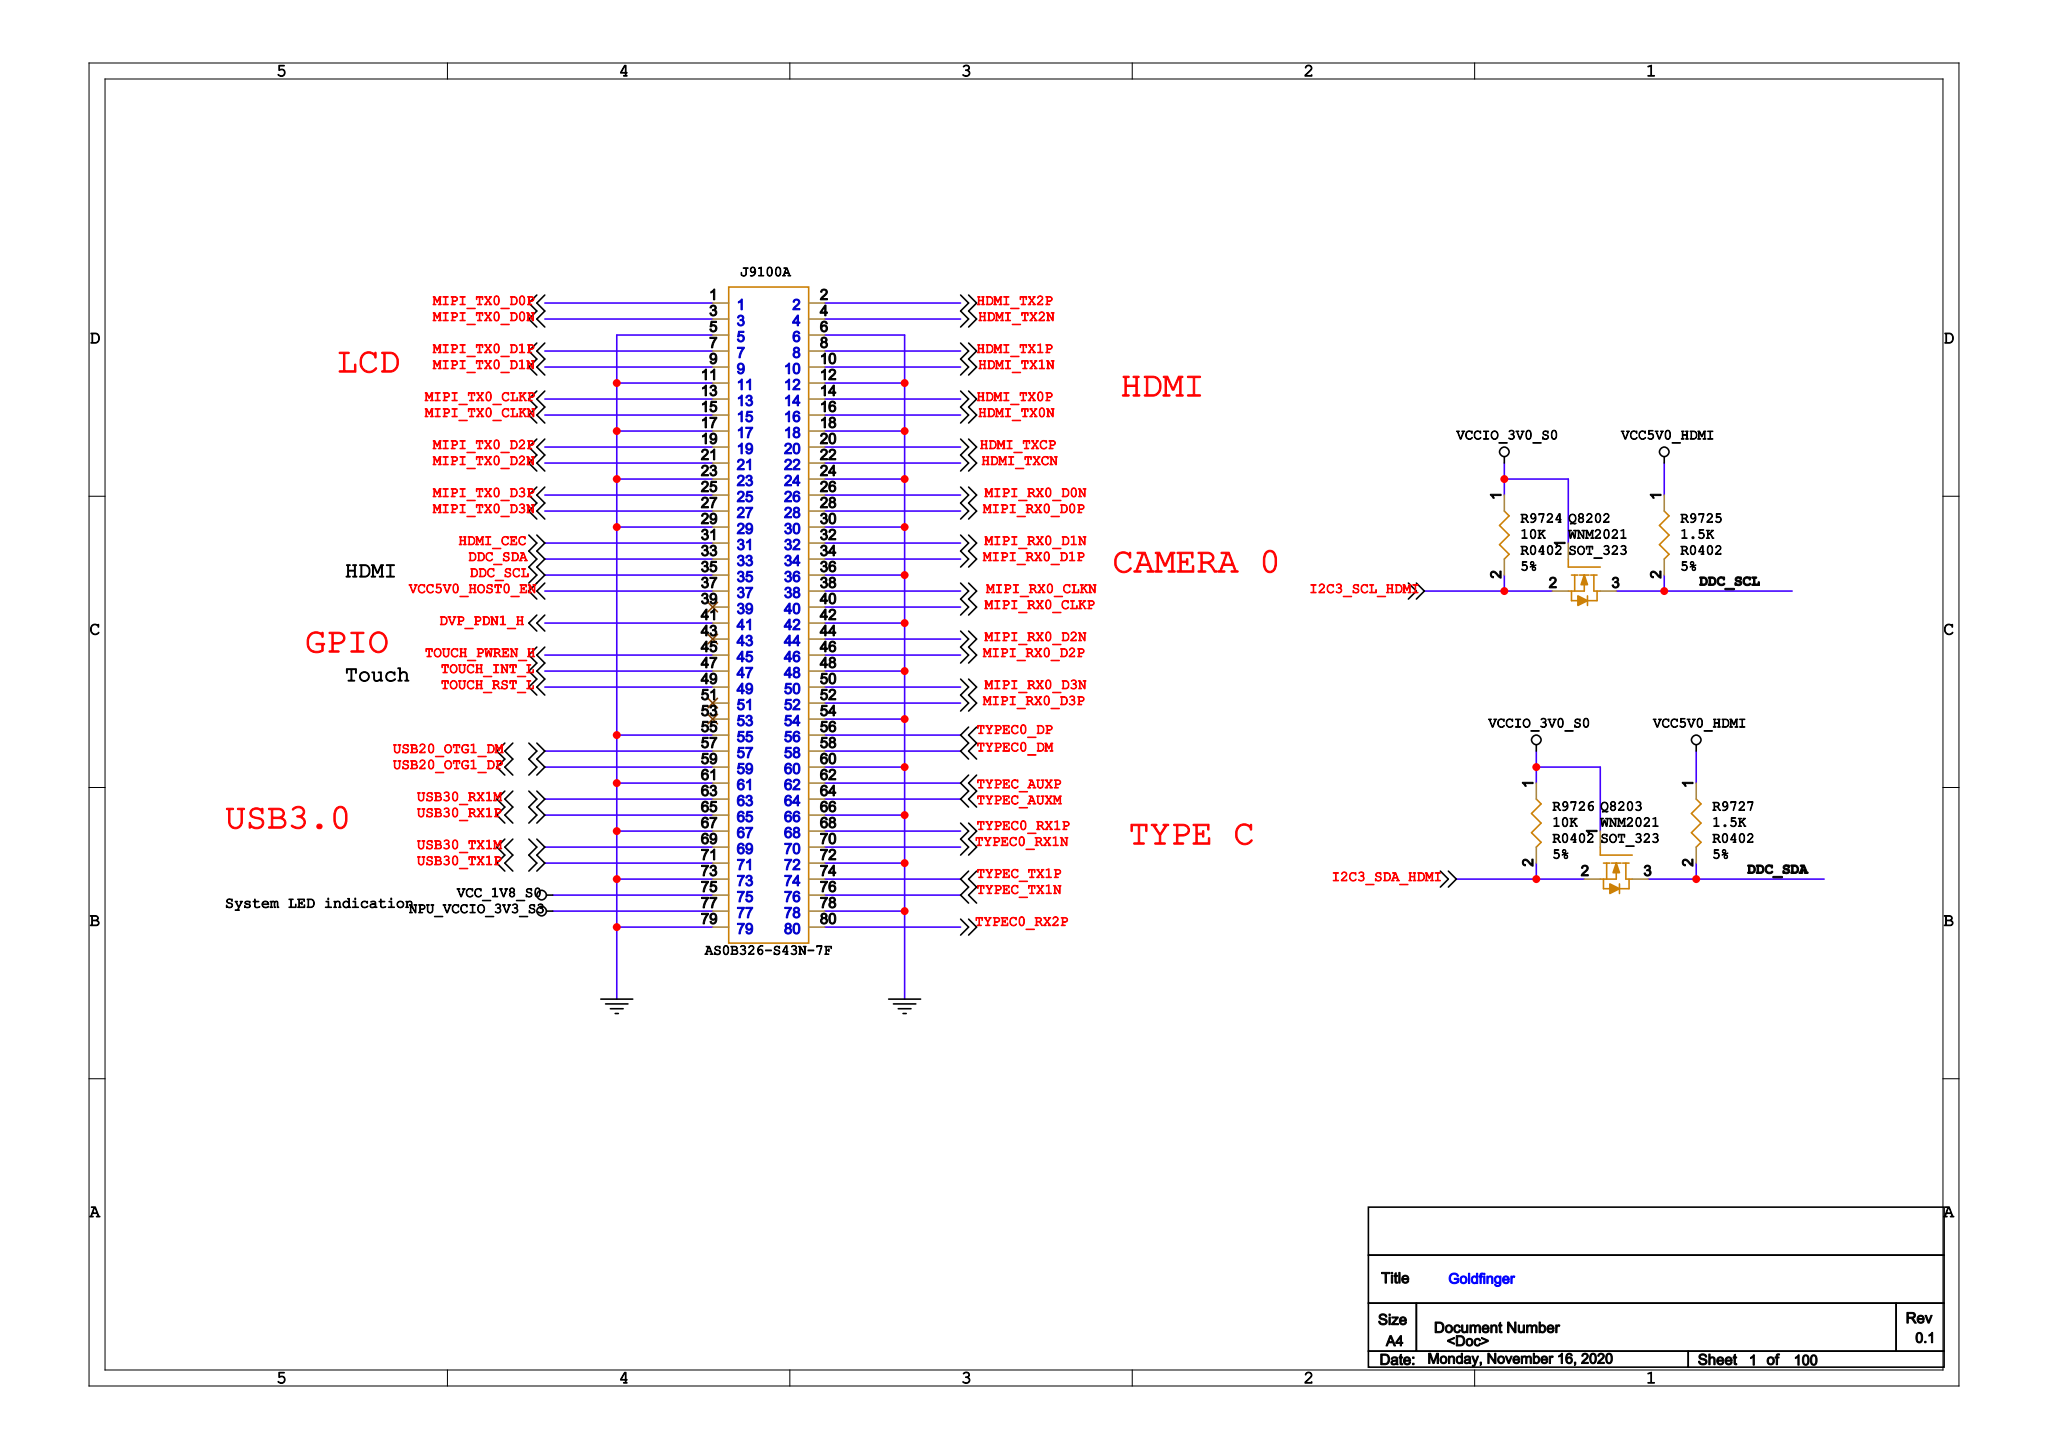Circuit board | Cadence Allegro | 749 parts | 717 nets | one sheet of the schematic
Parts on this sheet (reference | value | footprint):
J9100 | AS0B326-S43N-7F | MXM_230P_0P5
Q8202 | WNM2021 | SOT_323
Q8203 | WNM2021 | SOT_323
R9724 | 10K | R0402
R9725 | 1.5K | R0402
R9726 | 10K | R0402
R9727 | 1.5K | R0402
Nets of these parts (net: part-pin ...):
MIPI_TX0_D0P: J9100-1
HDMI_TX1N: J9100-10
MIPI_TX0_CLKP: J9100-13
HDMI_TX0P: J9100-14
MIPI_TX0_CLKN: J9100-15
HDMI_TX0N: J9100-16
MIPI_TX0_D2P: J9100-19
HDMI_TX2P: J9100-2
HDMI_TXCP: J9100-20
MIPI_TX0_D2N: J9100-21
HDMI_TXCN: J9100-22
MIPI_TX0_D3P: J9100-25
MIPI_RX0_D0N: J9100-26
MIPI_TX0_D3N: J9100-27
MIPI_RX0_D0P: J9100-28
MIPI_TX0_D0N: J9100-3
HDMI_CEC: J9100-31
MIPI_RX0_D1N: J9100-32
DDC_SDA: Q8203-3 R9727-2 J9100-33
MIPI_RX0_D1P: J9100-34
DDC_SCL: Q8202-3 R9725-2 J9100-35
VCC5V0_HOST0_EN: J9100-37
MIPI_RX0_CLKN: J9100-38
HDMI_TX2N: J9100-4
MIPI_RX0_CLKP: J9100-40
DVP_PDN1_H: J9100-41
MIPI_RX0_D2N: J9100-44
TOUCH_PWREN_H: J9100-45
MIPI_RX0_D2P: J9100-46
TOUCH_INT_L: J9100-47
TOUCH_RST_L: J9100-49
MIPI_RX0_D3N: J9100-50
MIPI_RX0_D3P: J9100-52
TYPEC0_DP: J9100-56
USB20_OTG1_DM: J9100-57
TYPEC0_DM: J9100-58
USB20_OTG1_DP: J9100-59
TYPEC_AUXP: J9100-62
USB30_RX1M: J9100-63
TYPEC_AUXM: J9100-64
USB30_RX1P: J9100-65
TYPEC0_RX1P: J9100-68
USB30_TX1M: J9100-69
MIPI_TX0_D1P: J9100-7
TYPEC0_RX1N: J9100-70
USB30_TX1P: J9100-71
TYPEC_TX1P: J9100-74
VCC_1V8_S0: J9100-75
TYPEC_TX1N: J9100-76
NPU_VCCIO_3V3_S3: J9100-77
HDMI_TX1P: J9100-8
TYPEC0_RX2P: J9100-80
MIPI_TX0_D1N: J9100-9
VCCIO_3V0_S0: Q8202-1 Q8203-1 R9724-1 R9726-1
I2C3_SCL_HDMI: Q8202-2 R9724-2
I2C3_SDA_HDMI: Q8203-2 R9726-2
VCC5V0_HDMI: R9725-1 R9727-1